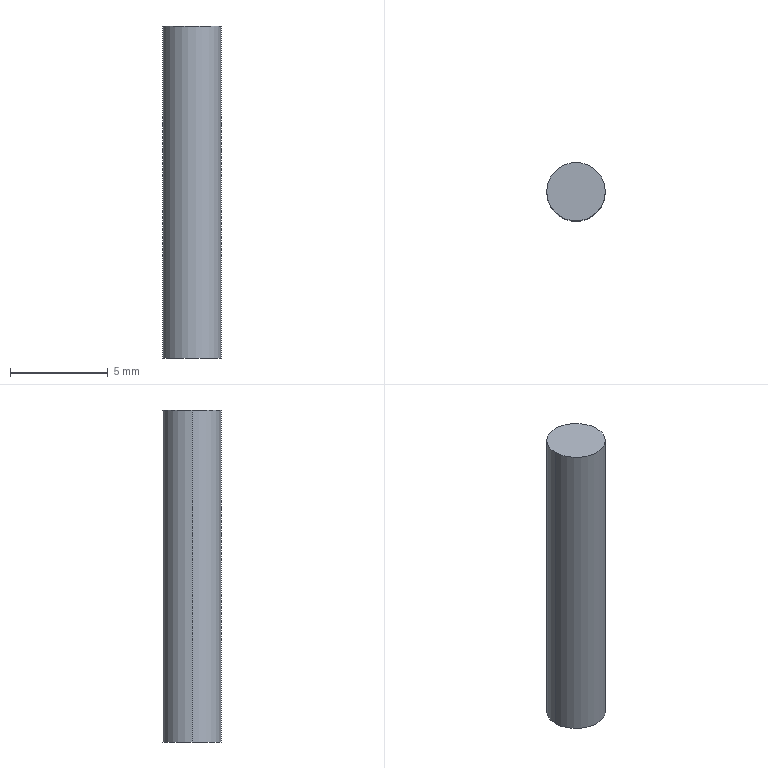Part | STEP file | Mount electronic clip pin shaft | 1 solid | 4 faces | box 3 x 3 x 17 mm | volume 120.166 mm3 | cylinder 2 | plane 2 | commonest cylinder face diameters 3 x2
STEP:
#1=CARTESIAN_POINT('',(0.,0.,0.));
#2=DIRECTION('',(0.,0.,1.));
#3=DIRECTION('',(1.,0.,0.));
#4=AXIS2_PLACEMENT_3D('',#1,#2,#3);
#5=CARTESIAN_POINT('',(1.5,0.,17.));
#6=VERTEX_POINT('',#5);
#7=CARTESIAN_POINT('',(-1.5,0.,17.));
#8=VERTEX_POINT('',#7);
#9=CARTESIAN_POINT('',(0.,0.,17.));
#10=DIRECTION('',(0.,0.,1.));
#11=DIRECTION('',(1.,0.,0.));
#12=AXIS2_PLACEMENT_3D('',#9,#10,#11);
#13=CIRCLE('',#12,1.5);
#14=CARTESIAN_POINT('',(0.,0.,17.));
#15=DIRECTION('',(0.,0.,-1.));
#16=DIRECTION('',(-1.,0.,0.));
#17=AXIS2_PLACEMENT_3D('',#14,#15,#16);
#18=CYLINDRICAL_SURFACE('',#17,1.5);
#19=CARTESIAN_POINT('',(3.142,0.));
#20=DIRECTION('',(-1.,0.));
#21=VECTOR('',#20,1.);
#22=LINE('',#19,#21);
#23=(GEOMETRIC_REPRESENTATION_CONTEXT(2)PARAMETRIC_REPRESENTATION_CONTEXT()REPRESENTATION_CONTEXT('',''));
#24=DEFINITIONAL_REPRESENTATION('',(#22),#23);
#25=PCURVE('',#18,#24);
#26=CARTESIAN_POINT('',(0.,0.,17.));
#27=DIRECTION('',(0.,0.,1.));
#28=DIRECTION('',(1.,0.,0.));
#29=AXIS2_PLACEMENT_3D('',#26,#27,#28);
#30=PLANE('',#29);
#31=CARTESIAN_POINT('',(0.,0.));
#32=DIRECTION('',(1.,0.));
#33=AXIS2_PLACEMENT_2D('',#31,#32);
#34=CIRCLE('',#33,1.5);
#35=(GEOMETRIC_REPRESENTATION_CONTEXT(2)PARAMETRIC_REPRESENTATION_CONTEXT()REPRESENTATION_CONTEXT('',''));
#36=DEFINITIONAL_REPRESENTATION('',(#34),#35);
#37=PCURVE('',#30,#36);
#38=SURFACE_CURVE('',#13,(#25,#37),.PCURVE_S1.);
#39=EDGE_CURVE('',#6,#8,#38,.T.);
#40=ORIENTED_EDGE('',*,*,#39,.F.);
#41=CARTESIAN_POINT('',(1.5,0.,0.));
#42=VERTEX_POINT('',#41);
#43=CARTESIAN_POINT('',(1.5,0.,17.));
#44=DIRECTION('',(0.,0.,-1.));
#45=VECTOR('',#44,1.);
#46=LINE('',#43,#45);
#47=CARTESIAN_POINT('',(3.142,0.));
#48=DIRECTION('',(0.,1.));
#49=VECTOR('',#48,1.);
#50=LINE('',#47,#49);
#51=(GEOMETRIC_REPRESENTATION_CONTEXT(2)PARAMETRIC_REPRESENTATION_CONTEXT()REPRESENTATION_CONTEXT('',''));
#52=DEFINITIONAL_REPRESENTATION('',(#50),#51);
#53=PCURVE('',#18,#52);
#54=CARTESIAN_POINT('',(0.,0.,17.));
#55=DIRECTION('',(0.,0.,-1.));
#56=DIRECTION('',(-1.,0.,0.));
#57=AXIS2_PLACEMENT_3D('',#54,#55,#56);
#58=CYLINDRICAL_SURFACE('',#57,1.5);
#59=CARTESIAN_POINT('',(3.142,0.));
#60=DIRECTION('',(0.,1.));
#61=VECTOR('',#60,1.);
#62=LINE('',#59,#61);
#63=(GEOMETRIC_REPRESENTATION_CONTEXT(2)PARAMETRIC_REPRESENTATION_CONTEXT()REPRESENTATION_CONTEXT('',''));
#64=DEFINITIONAL_REPRESENTATION('',(#62),#63);
#65=PCURVE('',#58,#64);
#66=SURFACE_CURVE('',#46,(#53,#65),.PCURVE_S1.);
#67=EDGE_CURVE('',#6,#42,#66,.T.);
#68=ORIENTED_EDGE('',*,*,#67,.T.);
#69=CARTESIAN_POINT('',(-1.5,0.,0.));
#70=VERTEX_POINT('',#69);
#71=CARTESIAN_POINT('',(0.,0.,0.));
#72=DIRECTION('',(0.,0.,1.));
#73=DIRECTION('',(1.,0.,0.));
#74=AXIS2_PLACEMENT_3D('',#71,#72,#73);
#75=CIRCLE('',#74,1.5);
#76=CARTESIAN_POINT('',(3.142,17.));
#77=DIRECTION('',(-1.,0.));
#78=VECTOR('',#77,1.);
#79=LINE('',#76,#78);
#80=(GEOMETRIC_REPRESENTATION_CONTEXT(2)PARAMETRIC_REPRESENTATION_CONTEXT()REPRESENTATION_CONTEXT('',''));
#81=DEFINITIONAL_REPRESENTATION('',(#79),#80);
#82=PCURVE('',#18,#81);
#83=CARTESIAN_POINT('',(0.,0.,0.));
#84=DIRECTION('',(0.,0.,1.));
#85=DIRECTION('',(1.,0.,0.));
#86=AXIS2_PLACEMENT_3D('',#83,#84,#85);
#87=PLANE('',#86);
#88=CARTESIAN_POINT('',(0.,0.));
#89=DIRECTION('',(1.,0.));
#90=AXIS2_PLACEMENT_2D('',#88,#89);
#91=CIRCLE('',#90,1.5);
#92=(GEOMETRIC_REPRESENTATION_CONTEXT(2)PARAMETRIC_REPRESENTATION_CONTEXT()REPRESENTATION_CONTEXT('',''));
#93=DEFINITIONAL_REPRESENTATION('',(#91),#92);
#94=PCURVE('',#87,#93);
#95=SURFACE_CURVE('',#75,(#82,#94),.PCURVE_S1.);
#96=EDGE_CURVE('',#42,#70,#95,.T.);
#97=ORIENTED_EDGE('',*,*,#96,.T.);
#98=CARTESIAN_POINT('',(-1.5,0.,17.));
#99=DIRECTION('',(0.,0.,-1.));
#100=VECTOR('',#99,1.);
#101=LINE('',#98,#100);
#102=CARTESIAN_POINT('',(0.,0.));
#103=DIRECTION('',(0.,1.));
#104=VECTOR('',#103,1.);
#105=LINE('',#102,#104);
#106=(GEOMETRIC_REPRESENTATION_CONTEXT(2)PARAMETRIC_REPRESENTATION_CONTEXT()REPRESENTATION_CONTEXT('',''));
#107=DEFINITIONAL_REPRESENTATION('',(#105),#106);
#108=PCURVE('',#18,#107);
#109=CARTESIAN_POINT('',(6.283,0.));
#110=DIRECTION('',(0.,1.));
#111=VECTOR('',#110,1.);
#112=LINE('',#109,#111);
#113=(GEOMETRIC_REPRESENTATION_CONTEXT(2)PARAMETRIC_REPRESENTATION_CONTEXT()REPRESENTATION_CONTEXT('',''));
#114=DEFINITIONAL_REPRESENTATION('',(#112),#113);
#115=PCURVE('',#58,#114);
#116=SURFACE_CURVE('',#101,(#108,#115),.PCURVE_S1.);
#117=EDGE_CURVE('',#8,#70,#116,.T.);
#118=ORIENTED_EDGE('',*,*,#117,.F.);
#119=EDGE_LOOP('',(#40,#68,#97,#118));
#120=FACE_BOUND('',#119,.T.);
#121=ADVANCED_FACE('',(#120),#18,.T.);
#122=ORIENTED_EDGE('',*,*,#67,.F.);
#123=CARTESIAN_POINT('',(0.,0.,17.));
#124=DIRECTION('',(0.,0.,1.));
#125=DIRECTION('',(1.,0.,0.));
#126=AXIS2_PLACEMENT_3D('',#123,#124,#125);
#127=CIRCLE('',#126,1.5);
#128=CARTESIAN_POINT('',(9.425,0.));
#129=DIRECTION('',(-1.,0.));
#130=VECTOR('',#129,1.);
#131=LINE('',#128,#130);
#132=(GEOMETRIC_REPRESENTATION_CONTEXT(2)PARAMETRIC_REPRESENTATION_CONTEXT()REPRESENTATION_CONTEXT('',''));
#133=DEFINITIONAL_REPRESENTATION('',(#131),#132);
#134=PCURVE('',#58,#133);
#135=CARTESIAN_POINT('',(0.,0.));
#136=DIRECTION('',(1.,0.));
#137=AXIS2_PLACEMENT_2D('',#135,#136);
#138=CIRCLE('',#137,1.5);
#139=(GEOMETRIC_REPRESENTATION_CONTEXT(2)PARAMETRIC_REPRESENTATION_CONTEXT()REPRESENTATION_CONTEXT('',''));
#140=DEFINITIONAL_REPRESENTATION('',(#138),#139);
#141=PCURVE('',#30,#140);
#142=SURFACE_CURVE('',#127,(#134,#141),.PCURVE_S1.);
#143=EDGE_CURVE('',#8,#6,#142,.T.);
#144=ORIENTED_EDGE('',*,*,#143,.F.);
#145=ORIENTED_EDGE('',*,*,#117,.T.);
#146=CARTESIAN_POINT('',(0.,0.,0.));
#147=DIRECTION('',(0.,0.,1.));
#148=DIRECTION('',(1.,0.,0.));
#149=AXIS2_PLACEMENT_3D('',#146,#147,#148);
#150=CIRCLE('',#149,1.5);
#151=CARTESIAN_POINT('',(9.425,17.));
#152=DIRECTION('',(-1.,0.));
#153=VECTOR('',#152,1.);
#154=LINE('',#151,#153);
#155=(GEOMETRIC_REPRESENTATION_CONTEXT(2)PARAMETRIC_REPRESENTATION_CONTEXT()REPRESENTATION_CONTEXT('',''));
#156=DEFINITIONAL_REPRESENTATION('',(#154),#155);
#157=PCURVE('',#58,#156);
#158=CARTESIAN_POINT('',(0.,0.));
#159=DIRECTION('',(1.,0.));
#160=AXIS2_PLACEMENT_2D('',#158,#159);
#161=CIRCLE('',#160,1.5);
#162=(GEOMETRIC_REPRESENTATION_CONTEXT(2)PARAMETRIC_REPRESENTATION_CONTEXT()REPRESENTATION_CONTEXT('',''));
#163=DEFINITIONAL_REPRESENTATION('',(#161),#162);
#164=PCURVE('',#87,#163);
#165=SURFACE_CURVE('',#150,(#157,#164),.PCURVE_S1.);
#166=EDGE_CURVE('',#70,#42,#165,.T.);
#167=ORIENTED_EDGE('',*,*,#166,.T.);
#168=EDGE_LOOP('',(#122,#144,#145,#167));
#169=FACE_BOUND('',#168,.T.);
#170=ADVANCED_FACE('',(#169),#58,.T.);
#171=ORIENTED_EDGE('',*,*,#143,.T.);
#172=ORIENTED_EDGE('',*,*,#39,.T.);
#173=EDGE_LOOP('',(#171,#172));
#174=FACE_BOUND('',#173,.T.);
#175=ADVANCED_FACE('',(#174),#30,.T.);
#176=ORIENTED_EDGE('',*,*,#166,.F.);
#177=ORIENTED_EDGE('',*,*,#96,.F.);
#178=EDGE_LOOP('',(#176,#177));
#179=FACE_BOUND('',#178,.T.);
#180=ADVANCED_FACE('',(#179),#87,.F.);
#181=CLOSED_SHELL('',(#121,#170,#175,#180));
#182=MANIFOLD_SOLID_BREP('',#181);
#183=(LENGTH_UNIT()NAMED_UNIT(*)SI_UNIT(.MILLI.,.METRE.));
#184=UNCERTAINTY_MEASURE_WITH_UNIT(LENGTH_MEASURE(0.0000001),#183,'','');
#185=(NAMED_UNIT(*)PLANE_ANGLE_UNIT()SI_UNIT($,.RADIAN.));
#186=(NAMED_UNIT(*)SI_UNIT($,.STERADIAN.)SOLID_ANGLE_UNIT());
#187=(GEOMETRIC_REPRESENTATION_CONTEXT(3)GLOBAL_UNCERTAINTY_ASSIGNED_CONTEXT((#184))GLOBAL_UNIT_ASSIGNED_CONTEXT((#183,#185,#186))REPRESENTATION_CONTEXT('',''));
#188=ADVANCED_BREP_SHAPE_REPRESENTATION('',(#4,#182),#187);